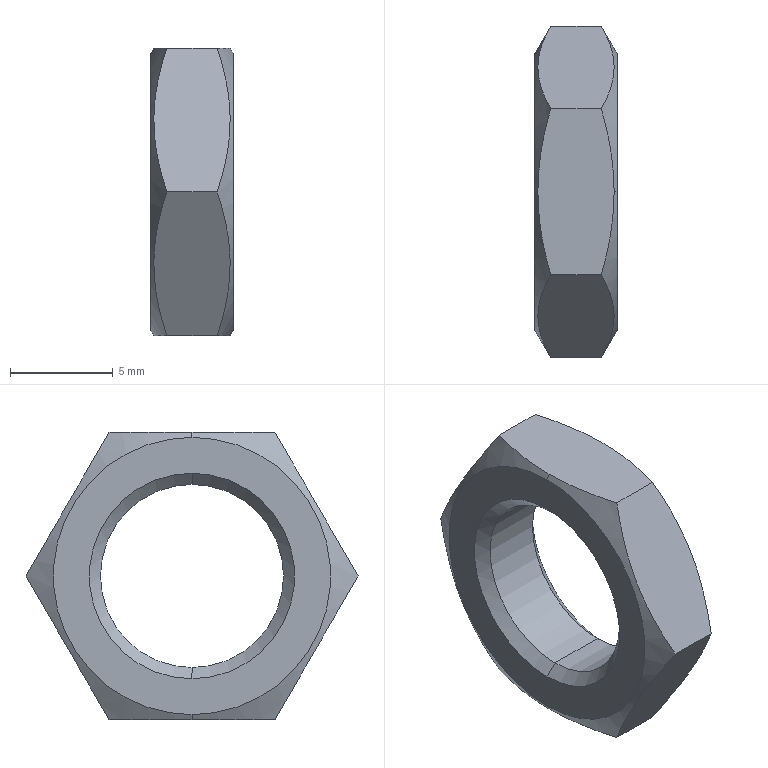Part | SolidWorks | features BaseBody 1 | 1 solid | 18 faces | box 4 x 16.166 x 14 mm | volume 408.53 mm3 | cone 8 | plane 8 | cylinder 2 | commonest cylinder face diameters 8.917 x2
STEP:
#1=CARTESIAN_POINT('',(-2.842,0.,4.458));
#2=VERTEX_POINT('',#1);
#3=CARTESIAN_POINT('',(-2.842,0.,-4.458));
#4=VERTEX_POINT('',#3);
#5=CARTESIAN_POINT('',(-2.842,0.,0.));
#6=DIRECTION('',(1.,0.,0.));
#7=DIRECTION('',(0.,1.,0.));
#8=AXIS2_PLACEMENT_3D('',#5,#6,#7);
#9=CIRCLE('',#8,4.458);
#10=EDGE_CURVE('',#2,#4,#9,.T.);
#11=ORIENTED_EDGE('',*,*,#10,.F.);
#12=CARTESIAN_POINT('',(-2.3,0.,5.));
#13=VERTEX_POINT('',#12);
#14=CARTESIAN_POINT('',(-2.3,0.,5.));
#15=DIRECTION('',(0.7071,0.,0.7071));
#16=VECTOR('',#15,1000.);
#17=LINE('',#14,#16);
#18=EDGE_CURVE('',#2,#13,#17,.T.);
#19=ORIENTED_EDGE('',*,*,#18,.T.);
#20=CARTESIAN_POINT('',(-2.3,0.,-5.));
#21=VERTEX_POINT('',#20);
#22=CARTESIAN_POINT('',(-2.3,0.,0.));
#23=DIRECTION('',(-1.,0.,0.));
#24=DIRECTION('',(0.,0.,-1.));
#25=AXIS2_PLACEMENT_3D('',#22,#23,#24);
#26=CIRCLE('',#25,5.);
#27=EDGE_CURVE('',#21,#13,#26,.T.);
#28=ORIENTED_EDGE('',*,*,#27,.F.);
#29=CARTESIAN_POINT('',(-2.3,0.,-5.));
#30=DIRECTION('',(0.7071,0.,-0.7071));
#31=VECTOR('',#30,1000.);
#32=LINE('',#29,#31);
#33=EDGE_CURVE('',#4,#21,#32,.T.);
#34=ORIENTED_EDGE('',*,*,#33,.F.);
#35=EDGE_LOOP('',(#11,#19,#28,#34));
#36=FACE_OUTER_BOUND('',#35,.T.);
#37=CARTESIAN_POINT('',(-2.3,0.,0.));
#38=DIRECTION('',(1.,0.,0.));
#39=DIRECTION('',(0.,0.,-1.));
#40=AXIS2_PLACEMENT_3D('',#37,#38,#39);
#41=CONICAL_SURFACE('',#40,5.,0.7854);
#42=ADVANCED_FACE('',(#36),#41,.F.);
#43=CARTESIAN_POINT('',(-2.3,0.,-6.75));
#44=VERTEX_POINT('',#43);
#45=CARTESIAN_POINT('',(-2.3,0.,6.75));
#46=VERTEX_POINT('',#45);
#47=CARTESIAN_POINT('',(-2.3,0.,0.));
#48=DIRECTION('',(1.,0.,0.));
#49=DIRECTION('',(0.,0.,1.));
#50=AXIS2_PLACEMENT_3D('',#47,#48,#49);
#51=CIRCLE('',#50,6.75);
#52=EDGE_CURVE('',#44,#46,#51,.T.);
#53=ORIENTED_EDGE('',*,*,#52,.F.);
#54=CARTESIAN_POINT('',(-2.444,0.,-7.));
#55=VERTEX_POINT('',#54);
#56=CARTESIAN_POINT('',(-3.074,0.,-8.091));
#57=DIRECTION('',(-0.5,0.,-0.866));
#58=VECTOR('',#57,1000.);
#59=LINE('',#56,#58);
#60=EDGE_CURVE('',#44,#55,#59,.T.);
#61=ORIENTED_EDGE('',*,*,#60,.T.);
#62=CARTESIAN_POINT('',(-3.07,4.041,-7.));
#63=VERTEX_POINT('',#62);
#64=CARTESIAN_POINT('',(-2.444,0.,-7.));
#65=CARTESIAN_POINT('',(-2.444,0.343,-7.));
#66=CARTESIAN_POINT('',(-2.459,0.6875,-7.));
#67=CARTESIAN_POINT('',(-2.516,1.369,-7.));
#68=CARTESIAN_POINT('',(-2.559,1.708,-7.));
#69=CARTESIAN_POINT('',(-2.722,2.717,-7.));
#70=CARTESIAN_POINT('',(-2.879,3.382,-7.));
#71=CARTESIAN_POINT('',(-3.07,4.041,-7.));
#72=B_SPLINE_CURVE_WITH_KNOTS('',3,(#64,#65,#66,#67,#68,#69,#70,#71),.UNSPECIFIED.,.F.,.F.,(4,2,2,4),(0.004089,0.005108,0.006126,0.008163),.UNSPECIFIED.);
#73=EDGE_CURVE('',#55,#63,#72,.T.);
#74=ORIENTED_EDGE('',*,*,#73,.T.);
#75=CARTESIAN_POINT('',(-3.07,8.083,0.));
#76=VERTEX_POINT('',#75);
#77=CARTESIAN_POINT('',(-3.07,4.041,-7.));
#78=CARTESIAN_POINT('',(-2.879,4.371,-6.429));
#79=CARTESIAN_POINT('',(-2.722,4.704,-5.853));
#80=CARTESIAN_POINT('',(-2.505,5.375,-4.69));
#81=CARTESIAN_POINT('',(-2.445,5.715,-4.102));
#82=CARTESIAN_POINT('',(-2.444,6.23,-3.209));
#83=CARTESIAN_POINT('',(-2.459,6.403,-2.91));
#84=CARTESIAN_POINT('',(-2.516,6.744,-2.319));
#85=CARTESIAN_POINT('',(-2.558,6.914,-2.025));
#86=CARTESIAN_POINT('',(-2.721,7.419,-1.149));
#87=CARTESIAN_POINT('',(-2.879,7.753,-0.5722));
#88=CARTESIAN_POINT('',(-3.07,8.083,0.));
#89=B_SPLINE_CURVE_WITH_KNOTS('',3,(#77,#78,#79,#80,#81,#82,#83,#84,#85,#86,#87,#88),.UNSPECIFIED.,.F.,.F.,(4,2,2,2,2,4),(0.,0.002041,0.004082,0.005102,0.006122,0.008163),.UNSPECIFIED.);
#90=EDGE_CURVE('',#63,#76,#89,.T.);
#91=ORIENTED_EDGE('',*,*,#90,.T.);
#92=CARTESIAN_POINT('',(-3.07,4.041,7.));
#93=VERTEX_POINT('',#92);
#94=CARTESIAN_POINT('',(-3.07,8.083,0.));
#95=CARTESIAN_POINT('',(-2.879,7.753,0.5715));
#96=CARTESIAN_POINT('',(-2.722,7.421,1.147));
#97=CARTESIAN_POINT('',(-2.505,6.749,2.31));
#98=CARTESIAN_POINT('',(-2.445,6.41,2.898));
#99=CARTESIAN_POINT('',(-2.444,5.894,3.791));
#100=CARTESIAN_POINT('',(-2.459,5.722,4.09));
#101=CARTESIAN_POINT('',(-2.516,5.38,4.681));
#102=CARTESIAN_POINT('',(-2.558,5.211,4.975));
#103=CARTESIAN_POINT('',(-2.721,4.705,5.851));
#104=CARTESIAN_POINT('',(-2.879,4.372,6.428));
#105=CARTESIAN_POINT('',(-3.07,4.041,7.));
#106=B_SPLINE_CURVE_WITH_KNOTS('',3,(#94,#95,#96,#97,#98,#99,#100,#101,#102,#103,#104,#105),.UNSPECIFIED.,.F.,.F.,(4,2,2,2,2,4),(0.,0.002041,0.004082,0.005102,0.006122,0.008163),.UNSPECIFIED.);
#107=EDGE_CURVE('',#76,#93,#106,.T.);
#108=ORIENTED_EDGE('',*,*,#107,.T.);
#109=CARTESIAN_POINT('',(-2.444,0.,7.));
#110=VERTEX_POINT('',#109);
#111=CARTESIAN_POINT('',(-3.07,4.041,7.));
#112=CARTESIAN_POINT('',(-2.879,3.38,7.));
#113=CARTESIAN_POINT('',(-2.721,2.714,7.));
#114=CARTESIAN_POINT('',(-2.504,1.369,7.));
#115=CARTESIAN_POINT('',(-2.444,0.6885,7.));
#116=CARTESIAN_POINT('',(-2.444,0.,7.));
#117=B_SPLINE_CURVE_WITH_KNOTS('',3,(#111,#112,#113,#114,#115,#116),.UNSPECIFIED.,.F.,.F.,(4,2,4),(0.,0.002045,0.004089),.UNSPECIFIED.);
#118=EDGE_CURVE('',#93,#110,#117,.T.);
#119=ORIENTED_EDGE('',*,*,#118,.T.);
#120=CARTESIAN_POINT('',(-3.074,0.,8.091));
#121=DIRECTION('',(-0.5,0.,0.866));
#122=VECTOR('',#121,1000.);
#123=LINE('',#120,#122);
#124=EDGE_CURVE('',#46,#110,#123,.T.);
#125=ORIENTED_EDGE('',*,*,#124,.F.);
#126=EDGE_LOOP('',(#53,#61,#74,#91,#108,#119,#125));
#127=FACE_OUTER_BOUND('',#126,.T.);
#128=CARTESIAN_POINT('',(-3.074,0.,0.));
#129=DIRECTION('',(-1.,0.,0.));
#130=DIRECTION('',(0.,0.,1.));
#131=AXIS2_PLACEMENT_3D('',#128,#129,#130);
#132=CONICAL_SURFACE('',#131,8.091,1.047);
#133=ADVANCED_FACE('',(#127),#132,.T.);
#134=CARTESIAN_POINT('',(-5.758,0.,4.458));
#135=VERTEX_POINT('',#134);
#136=CARTESIAN_POINT('',(-5.758,0.,-4.458));
#137=VERTEX_POINT('',#136);
#138=CARTESIAN_POINT('',(-5.758,0.,0.));
#139=DIRECTION('',(1.,0.,0.));
#140=DIRECTION('',(0.,0.,-1.));
#141=AXIS2_PLACEMENT_3D('',#138,#139,#140);
#142=CIRCLE('',#141,4.458);
#143=EDGE_CURVE('',#135,#137,#142,.T.);
#144=ORIENTED_EDGE('',*,*,#143,.F.);
#145=CARTESIAN_POINT('',(-4.3,0.,4.458));
#146=DIRECTION('',(1.,0.,0.));
#147=VECTOR('',#146,1000.);
#148=LINE('',#145,#147);
#149=EDGE_CURVE('',#135,#2,#148,.T.);
#150=ORIENTED_EDGE('',*,*,#149,.T.);
#151=ORIENTED_EDGE('',*,*,#10,.T.);
#152=CARTESIAN_POINT('',(-4.3,0.,-4.458));
#153=DIRECTION('',(1.,0.,0.));
#154=VECTOR('',#153,1000.);
#155=LINE('',#152,#154);
#156=EDGE_CURVE('',#137,#4,#155,.T.);
#157=ORIENTED_EDGE('',*,*,#156,.F.);
#158=EDGE_LOOP('',(#144,#150,#151,#157));
#159=FACE_OUTER_BOUND('',#158,.T.);
#160=CARTESIAN_POINT('',(-4.3,0.,0.));
#161=DIRECTION('',(1.,0.,0.));
#162=DIRECTION('',(0.,0.,-1.));
#163=AXIS2_PLACEMENT_3D('',#160,#161,#162);
#164=CYLINDRICAL_SURFACE('',#163,4.458);
#165=ADVANCED_FACE('',(#159),#164,.F.);
#166=ORIENTED_EDGE('',*,*,#143,.T.);
#167=CARTESIAN_POINT('',(-6.3,0.,-5.));
#168=VERTEX_POINT('',#167);
#169=CARTESIAN_POINT('',(-6.3,0.,-5.));
#170=DIRECTION('',(-0.7071,0.,-0.7071));
#171=VECTOR('',#170,1000.);
#172=LINE('',#169,#171);
#173=EDGE_CURVE('',#137,#168,#172,.T.);
#174=ORIENTED_EDGE('',*,*,#173,.T.);
#175=CARTESIAN_POINT('',(-6.3,0.,5.));
#176=VERTEX_POINT('',#175);
#177=CARTESIAN_POINT('',(-6.3,0.,0.));
#178=DIRECTION('',(1.,0.,0.));
#179=DIRECTION('',(0.,0.,1.));
#180=AXIS2_PLACEMENT_3D('',#177,#178,#179);
#181=CIRCLE('',#180,5.);
#182=EDGE_CURVE('',#176,#168,#181,.T.);
#183=ORIENTED_EDGE('',*,*,#182,.F.);
#184=CARTESIAN_POINT('',(-6.3,0.,5.));
#185=DIRECTION('',(-0.7071,0.,0.7071));
#186=VECTOR('',#185,1000.);
#187=LINE('',#184,#186);
#188=EDGE_CURVE('',#135,#176,#187,.T.);
#189=ORIENTED_EDGE('',*,*,#188,.F.);
#190=EDGE_LOOP('',(#166,#174,#183,#189));
#191=FACE_OUTER_BOUND('',#190,.T.);
#192=CARTESIAN_POINT('',(-6.3,0.,0.));
#193=DIRECTION('',(-1.,0.,0.));
#194=DIRECTION('',(0.,0.,1.));
#195=AXIS2_PLACEMENT_3D('',#192,#193,#194);
#196=CONICAL_SURFACE('',#195,5.,0.7854);
#197=ADVANCED_FACE('',(#191),#196,.F.);
#198=CARTESIAN_POINT('',(-6.3,0.,-6.75));
#199=VERTEX_POINT('',#198);
#200=CARTESIAN_POINT('',(-6.3,0.,6.75));
#201=VERTEX_POINT('',#200);
#202=CARTESIAN_POINT('',(-6.3,0.,0.));
#203=DIRECTION('',(1.,0.,0.));
#204=DIRECTION('',(0.,0.,-1.));
#205=AXIS2_PLACEMENT_3D('',#202,#203,#204);
#206=CIRCLE('',#205,6.75);
#207=EDGE_CURVE('',#199,#201,#206,.T.);
#208=ORIENTED_EDGE('',*,*,#207,.T.);
#209=CARTESIAN_POINT('',(-6.156,0.,7.));
#210=VERTEX_POINT('',#209);
#211=CARTESIAN_POINT('',(-5.526,0.,8.091));
#212=DIRECTION('',(0.5,0.,0.866));
#213=VECTOR('',#212,1000.);
#214=LINE('',#211,#213);
#215=EDGE_CURVE('',#201,#210,#214,.T.);
#216=ORIENTED_EDGE('',*,*,#215,.T.);
#217=CARTESIAN_POINT('',(-5.53,4.041,7.));
#218=VERTEX_POINT('',#217);
#219=CARTESIAN_POINT('',(-5.53,4.041,7.));
#220=CARTESIAN_POINT('',(-5.721,3.38,7.));
#221=CARTESIAN_POINT('',(-5.879,2.714,7.));
#222=CARTESIAN_POINT('',(-6.096,1.369,7.));
#223=CARTESIAN_POINT('',(-6.156,0.6885,7.));
#224=CARTESIAN_POINT('',(-6.156,0.,7.));
#225=B_SPLINE_CURVE_WITH_KNOTS('',3,(#219,#220,#221,#222,#223,#224),.UNSPECIFIED.,.F.,.F.,(4,2,4),(0.,0.002045,0.004089),.UNSPECIFIED.);
#226=EDGE_CURVE('',#218,#210,#225,.T.);
#227=ORIENTED_EDGE('',*,*,#226,.F.);
#228=CARTESIAN_POINT('',(-5.53,8.083,0.));
#229=VERTEX_POINT('',#228);
#230=CARTESIAN_POINT('',(-5.53,8.083,0.));
#231=CARTESIAN_POINT('',(-5.721,7.753,0.5715));
#232=CARTESIAN_POINT('',(-5.878,7.421,1.147));
#233=CARTESIAN_POINT('',(-6.095,6.749,2.31));
#234=CARTESIAN_POINT('',(-6.155,6.41,2.898));
#235=CARTESIAN_POINT('',(-6.156,5.894,3.791));
#236=CARTESIAN_POINT('',(-6.141,5.722,4.09));
#237=CARTESIAN_POINT('',(-6.084,5.38,4.681));
#238=CARTESIAN_POINT('',(-6.042,5.211,4.975));
#239=CARTESIAN_POINT('',(-5.879,4.705,5.851));
#240=CARTESIAN_POINT('',(-5.721,4.372,6.428));
#241=CARTESIAN_POINT('',(-5.53,4.041,7.));
#242=B_SPLINE_CURVE_WITH_KNOTS('',3,(#230,#231,#232,#233,#234,#235,#236,#237,#238,#239,#240,#241),.UNSPECIFIED.,.F.,.F.,(4,2,2,2,2,4),(0.,0.002041,0.004082,0.005102,0.006122,0.008163),.UNSPECIFIED.);
#243=EDGE_CURVE('',#229,#218,#242,.T.);
#244=ORIENTED_EDGE('',*,*,#243,.F.);
#245=CARTESIAN_POINT('',(-5.53,4.041,-7.));
#246=VERTEX_POINT('',#245);
#247=CARTESIAN_POINT('',(-5.53,4.041,-7.));
#248=CARTESIAN_POINT('',(-5.721,4.371,-6.429));
#249=CARTESIAN_POINT('',(-5.878,4.704,-5.853));
#250=CARTESIAN_POINT('',(-6.095,5.375,-4.69));
#251=CARTESIAN_POINT('',(-6.155,5.715,-4.102));
#252=CARTESIAN_POINT('',(-6.156,6.23,-3.209));
#253=CARTESIAN_POINT('',(-6.141,6.403,-2.91));
#254=CARTESIAN_POINT('',(-6.084,6.744,-2.319));
#255=CARTESIAN_POINT('',(-6.042,6.914,-2.025));
#256=CARTESIAN_POINT('',(-5.879,7.419,-1.149));
#257=CARTESIAN_POINT('',(-5.721,7.753,-0.5722));
#258=CARTESIAN_POINT('',(-5.53,8.083,0.));
#259=B_SPLINE_CURVE_WITH_KNOTS('',3,(#247,#248,#249,#250,#251,#252,#253,#254,#255,#256,#257,#258),.UNSPECIFIED.,.F.,.F.,(4,2,2,2,2,4),(0.,0.002041,0.004082,0.005102,0.006122,0.008163),.UNSPECIFIED.);
#260=EDGE_CURVE('',#246,#229,#259,.T.);
#261=ORIENTED_EDGE('',*,*,#260,.F.);
#262=CARTESIAN_POINT('',(-6.156,0.,-7.));
#263=VERTEX_POINT('',#262);
#264=CARTESIAN_POINT('',(-6.156,0.,-7.));
#265=CARTESIAN_POINT('',(-6.156,0.343,-7.));
#266=CARTESIAN_POINT('',(-6.141,0.6875,-7.));
#267=CARTESIAN_POINT('',(-6.084,1.369,-7.));
#268=CARTESIAN_POINT('',(-6.041,1.708,-7.));
#269=CARTESIAN_POINT('',(-5.878,2.717,-7.));
#270=CARTESIAN_POINT('',(-5.721,3.382,-7.));
#271=CARTESIAN_POINT('',(-5.53,4.041,-7.));
#272=B_SPLINE_CURVE_WITH_KNOTS('',3,(#264,#265,#266,#267,#268,#269,#270,#271),.UNSPECIFIED.,.F.,.F.,(4,2,2,4),(0.004089,0.005108,0.006126,0.008163),.UNSPECIFIED.);
#273=EDGE_CURVE('',#263,#246,#272,.T.);
#274=ORIENTED_EDGE('',*,*,#273,.F.);
#275=CARTESIAN_POINT('',(-5.526,0.,-8.091));
#276=DIRECTION('',(0.5,0.,-0.866));
#277=VECTOR('',#276,1000.);
#278=LINE('',#275,#277);
#279=EDGE_CURVE('',#199,#263,#278,.T.);
#280=ORIENTED_EDGE('',*,*,#279,.F.);
#281=EDGE_LOOP('',(#208,#216,#227,#244,#261,#274,#280));
#282=FACE_OUTER_BOUND('',#281,.T.);
#283=CARTESIAN_POINT('',(-5.526,0.,0.));
#284=DIRECTION('',(1.,0.,0.));
#285=DIRECTION('',(0.,0.,-1.));
#286=AXIS2_PLACEMENT_3D('',#283,#284,#285);
#287=CONICAL_SURFACE('',#286,8.091,1.047);
#288=ADVANCED_FACE('',(#282),#287,.T.);
#289=ORIENTED_EDGE('',*,*,#27,.T.);
#290=CARTESIAN_POINT('',(-2.3,0.,0.));
#291=DIRECTION('',(-1.,0.,0.));
#292=DIRECTION('',(0.,0.,-1.));
#293=AXIS2_PLACEMENT_3D('',#290,#291,#292);
#294=CIRCLE('',#293,5.);
#295=EDGE_CURVE('',#13,#21,#294,.T.);
#296=ORIENTED_EDGE('',*,*,#295,.T.);
#297=EDGE_LOOP('',(#289,#296));
#298=FACE_BOUND('',#297,.T.);
#299=CARTESIAN_POINT('',(-2.3,0.,0.));
#300=DIRECTION('',(1.,0.,0.));
#301=DIRECTION('',(0.,0.,1.));
#302=AXIS2_PLACEMENT_3D('',#299,#300,#301);
#303=CIRCLE('',#302,6.75);
#304=EDGE_CURVE('',#46,#44,#303,.T.);
#305=ORIENTED_EDGE('',*,*,#304,.T.);
#306=ORIENTED_EDGE('',*,*,#52,.T.);
#307=EDGE_LOOP('',(#305,#306));
#308=FACE_OUTER_BOUND('',#307,.T.);
#309=CARTESIAN_POINT('',(-2.3,0.,0.));
#310=DIRECTION('',(1.,0.,0.));
#311=DIRECTION('',(0.,0.,-1.));
#312=AXIS2_PLACEMENT_3D('',#309,#310,#311);
#313=PLANE('',#312);
#314=ADVANCED_FACE('',(#298,#308),#313,.T.);
#315=ORIENTED_EDGE('',*,*,#18,.F.);
#316=CARTESIAN_POINT('',(-2.842,0.,0.));
#317=DIRECTION('',(1.,0.,0.));
#318=DIRECTION('',(0.,1.,0.));
#319=AXIS2_PLACEMENT_3D('',#316,#317,#318);
#320=CIRCLE('',#319,4.458);
#321=EDGE_CURVE('',#4,#2,#320,.T.);
#322=ORIENTED_EDGE('',*,*,#321,.F.);
#323=ORIENTED_EDGE('',*,*,#33,.T.);
#324=ORIENTED_EDGE('',*,*,#295,.F.);
#325=EDGE_LOOP('',(#315,#322,#323,#324));
#326=FACE_OUTER_BOUND('',#325,.T.);
#327=CARTESIAN_POINT('',(-2.3,0.,0.));
#328=DIRECTION('',(1.,0.,0.));
#329=DIRECTION('',(0.,0.,-1.));
#330=AXIS2_PLACEMENT_3D('',#327,#328,#329);
#331=CONICAL_SURFACE('',#330,5.,0.7854);
#332=ADVANCED_FACE('',(#326),#331,.F.);
#333=ORIENTED_EDGE('',*,*,#60,.F.);
#334=ORIENTED_EDGE('',*,*,#304,.F.);
#335=ORIENTED_EDGE('',*,*,#124,.T.);
#336=CARTESIAN_POINT('',(-3.07,-4.041,7.));
#337=VERTEX_POINT('',#336);
#338=CARTESIAN_POINT('',(-2.444,0.,7.));
#339=CARTESIAN_POINT('',(-2.444,-0.343,7.));
#340=CARTESIAN_POINT('',(-2.459,-0.6875,7.));
#341=CARTESIAN_POINT('',(-2.516,-1.369,7.));
#342=CARTESIAN_POINT('',(-2.559,-1.708,7.));
#343=CARTESIAN_POINT('',(-2.722,-2.717,7.));
#344=CARTESIAN_POINT('',(-2.879,-3.382,7.));
#345=CARTESIAN_POINT('',(-3.07,-4.041,7.));
#346=B_SPLINE_CURVE_WITH_KNOTS('',3,(#338,#339,#340,#341,#342,#343,#344,#345),.UNSPECIFIED.,.F.,.F.,(4,2,2,4),(0.004089,0.005108,0.006126,0.008163),.UNSPECIFIED.);
#347=EDGE_CURVE('',#110,#337,#346,.T.);
#348=ORIENTED_EDGE('',*,*,#347,.T.);
#349=CARTESIAN_POINT('',(-3.07,-8.083,0.));
#350=VERTEX_POINT('',#349);
#351=CARTESIAN_POINT('',(-3.07,-4.041,7.));
#352=CARTESIAN_POINT('',(-2.879,-4.371,6.429));
#353=CARTESIAN_POINT('',(-2.722,-4.704,5.853));
#354=CARTESIAN_POINT('',(-2.505,-5.375,4.69));
#355=CARTESIAN_POINT('',(-2.445,-5.715,4.102));
#356=CARTESIAN_POINT('',(-2.444,-6.23,3.209));
#357=CARTESIAN_POINT('',(-2.459,-6.403,2.91));
#358=CARTESIAN_POINT('',(-2.516,-6.744,2.319));
#359=CARTESIAN_POINT('',(-2.558,-6.914,2.025));
#360=CARTESIAN_POINT('',(-2.721,-7.419,1.149));
#361=CARTESIAN_POINT('',(-2.879,-7.753,0.5722));
#362=CARTESIAN_POINT('',(-3.07,-8.083,0.));
#363=B_SPLINE_CURVE_WITH_KNOTS('',3,(#351,#352,#353,#354,#355,#356,#357,#358,#359,#360,#361,#362),.UNSPECIFIED.,.F.,.F.,(4,2,2,2,2,4),(0.,0.002041,0.004082,0.005102,0.006122,0.008163),.UNSPECIFIED.);
#364=EDGE_CURVE('',#337,#350,#363,.T.);
#365=ORIENTED_EDGE('',*,*,#364,.T.);
#366=CARTESIAN_POINT('',(-3.07,-4.041,-7.));
#367=VERTEX_POINT('',#366);
#368=CARTESIAN_POINT('',(-3.07,-8.083,0.));
#369=CARTESIAN_POINT('',(-2.879,-7.753,-0.5715));
#370=CARTESIAN_POINT('',(-2.722,-7.421,-1.147));
#371=CARTESIAN_POINT('',(-2.505,-6.749,-2.31));
#372=CARTESIAN_POINT('',(-2.445,-6.41,-2.898));
#373=CARTESIAN_POINT('',(-2.444,-5.894,-3.791));
#374=CARTESIAN_POINT('',(-2.459,-5.722,-4.09));
#375=CARTESIAN_POINT('',(-2.516,-5.38,-4.681));
#376=CARTESIAN_POINT('',(-2.558,-5.211,-4.975));
#377=CARTESIAN_POINT('',(-2.721,-4.705,-5.851));
#378=CARTESIAN_POINT('',(-2.879,-4.372,-6.428));
#379=CARTESIAN_POINT('',(-3.07,-4.041,-7.));
#380=B_SPLINE_CURVE_WITH_KNOTS('',3,(#368,#369,#370,#371,#372,#373,#374,#375,#376,#377,#378,#379),.UNSPECIFIED.,.F.,.F.,(4,2,2,2,2,4),(0.,0.002041,0.004082,0.005102,0.006122,0.008163),.UNSPECIFIED.);
#381=EDGE_CURVE('',#350,#367,#380,.T.);
#382=ORIENTED_EDGE('',*,*,#381,.T.);
#383=CARTESIAN_POINT('',(-3.07,-4.041,-7.));
#384=CARTESIAN_POINT('',(-2.879,-3.38,-7.));
#385=CARTESIAN_POINT('',(-2.721,-2.714,-7.));
#386=CARTESIAN_POINT('',(-2.504,-1.369,-7.));
#387=CARTESIAN_POINT('',(-2.444,-0.6885,-7.));
#388=CARTESIAN_POINT('',(-2.444,0.,-7.));
#389=B_SPLINE_CURVE_WITH_KNOTS('',3,(#383,#384,#385,#386,#387,#388),.UNSPECIFIED.,.F.,.F.,(4,2,4),(0.,0.002045,0.004089),.UNSPECIFIED.);
#390=EDGE_CURVE('',#367,#55,#389,.T.);
#391=ORIENTED_EDGE('',*,*,#390,.T.);
#392=EDGE_LOOP('',(#333,#334,#335,#348,#365,#382,#391));
#393=FACE_OUTER_BOUND('',#392,.T.);
#394=CARTESIAN_POINT('',(-3.074,0.,0.));
#395=DIRECTION('',(-1.,0.,0.));
#396=DIRECTION('',(0.,0.,1.));
#397=AXIS2_PLACEMENT_3D('',#394,#395,#396);
#398=CONICAL_SURFACE('',#397,8.091,1.047);
#399=ADVANCED_FACE('',(#393),#398,.T.);
#400=ORIENTED_EDGE('',*,*,#149,.F.);
#401=CARTESIAN_POINT('',(-5.758,0.,0.));
#402=DIRECTION('',(1.,0.,0.));
#403=DIRECTION('',(0.,0.,-1.));
#404=AXIS2_PLACEMENT_3D('',#401,#402,#403);
#405=CIRCLE('',#404,4.458);
#406=EDGE_CURVE('',#137,#135,#405,.T.);
#407=ORIENTED_EDGE('',*,*,#406,.F.);
#408=ORIENTED_EDGE('',*,*,#156,.T.);
#409=ORIENTED_EDGE('',*,*,#321,.T.);
#410=EDGE_LOOP('',(#400,#407,#408,#409));
#411=FACE_OUTER_BOUND('',#410,.T.);
#412=CARTESIAN_POINT('',(-4.3,0.,0.));
#413=DIRECTION('',(1.,0.,0.));
#414=DIRECTION('',(0.,0.,-1.));
#415=AXIS2_PLACEMENT_3D('',#412,#413,#414);
#416=CYLINDRICAL_SURFACE('',#415,4.458);
#417=ADVANCED_FACE('',(#411),#416,.F.);
#418=ORIENTED_EDGE('',*,*,#90,.F.);
#419=CARTESIAN_POINT('',(-2.3,4.041,-7.));
#420=DIRECTION('',(-1.,0.,0.));
#421=VECTOR('',#420,1000.);
#422=LINE('',#419,#421);
#423=EDGE_CURVE('',#63,#246,#422,.T.);
#424=ORIENTED_EDGE('',*,*,#423,.T.);
#425=ORIENTED_EDGE('',*,*,#260,.T.);
#426=CARTESIAN_POINT('',(-2.3,8.083,0.));
#427=DIRECTION('',(1.,0.,0.));
#428=VECTOR('',#427,1000.);
#429=LINE('',#426,#428);
#430=EDGE_CURVE('',#229,#76,#429,.T.);
#431=ORIENTED_EDGE('',*,*,#430,.T.);
#432=EDGE_LOOP('',(#418,#424,#425,#431));
#433=FACE_OUTER_BOUND('',#432,.T.);
#434=CARTESIAN_POINT('',(-2.3,4.041,-7.));
#435=DIRECTION('',(0.,0.866,-0.5));
#436=DIRECTION('',(0.,0.5,0.866));
#437=AXIS2_PLACEMENT_3D('',#434,#435,#436);
#438=PLANE('',#437);
#439=ADVANCED_FACE('',(#433),#438,.T.);
#440=ORIENTED_EDGE('',*,*,#390,.F.);
#441=CARTESIAN_POINT('',(-5.53,-4.041,-7.));
#442=VERTEX_POINT('',#441);
#443=CARTESIAN_POINT('',(-2.3,-4.041,-7.));
#444=DIRECTION('',(-1.,0.,0.));
#445=VECTOR('',#444,1000.);
#446=LINE('',#443,#445);
#447=EDGE_CURVE('',#367,#442,#446,.T.);
#448=ORIENTED_EDGE('',*,*,#447,.T.);
#449=CARTESIAN_POINT('',(-5.53,-4.041,-7.));
#450=CARTESIAN_POINT('',(-5.721,-3.38,-7.));
#451=CARTESIAN_POINT('',(-5.879,-2.714,-7.));
#452=CARTESIAN_POINT('',(-6.096,-1.369,-7.));
#453=CARTESIAN_POINT('',(-6.156,-0.6885,-7.));
#454=CARTESIAN_POINT('',(-6.156,0.,-7.));
#455=B_SPLINE_CURVE_WITH_KNOTS('',3,(#449,#450,#451,#452,#453,#454),.UNSPECIFIED.,.F.,.F.,(4,2,4),(0.,0.002045,0.004089),.UNSPECIFIED.);
#456=EDGE_CURVE('',#442,#263,#455,.T.);
#457=ORIENTED_EDGE('',*,*,#456,.T.);
#458=ORIENTED_EDGE('',*,*,#273,.T.);
#459=ORIENTED_EDGE('',*,*,#423,.F.);
#460=ORIENTED_EDGE('',*,*,#73,.F.);
#461=EDGE_LOOP('',(#440,#448,#457,#458,#459,#460));
#462=FACE_OUTER_BOUND('',#461,.T.);
#463=CARTESIAN_POINT('',(-2.3,-4.041,-7.));
#464=DIRECTION('',(0.,0.,-1.));
#465=DIRECTION('',(-1.,0.,0.));
#466=AXIS2_PLACEMENT_3D('',#463,#464,#465);
#467=PLANE('',#466);
#468=ADVANCED_FACE('',(#462),#467,.T.);
#469=ORIENTED_EDGE('',*,*,#381,.F.);
#470=CARTESIAN_POINT('',(-5.53,-8.083,0.));
#471=VERTEX_POINT('',#470);
#472=CARTESIAN_POINT('',(-2.3,-8.083,0.));
#473=DIRECTION('',(-1.,0.,0.));
#474=VECTOR('',#473,1000.);
#475=LINE('',#472,#474);
#476=EDGE_CURVE('',#350,#471,#475,.T.);
#477=ORIENTED_EDGE('',*,*,#476,.T.);
#478=CARTESIAN_POINT('',(-5.53,-8.083,0.));
#479=CARTESIAN_POINT('',(-5.721,-7.753,-0.5715));
#480=CARTESIAN_POINT('',(-5.878,-7.421,-1.147));
#481=CARTESIAN_POINT('',(-6.095,-6.749,-2.31));
#482=CARTESIAN_POINT('',(-6.155,-6.41,-2.898));
#483=CARTESIAN_POINT('',(-6.156,-5.894,-3.791));
#484=CARTESIAN_POINT('',(-6.141,-5.722,-4.09));
#485=CARTESIAN_POINT('',(-6.084,-5.38,-4.681));
#486=CARTESIAN_POINT('',(-6.042,-5.211,-4.975));
#487=CARTESIAN_POINT('',(-5.879,-4.705,-5.851));
#488=CARTESIAN_POINT('',(-5.721,-4.372,-6.428));
#489=CARTESIAN_POINT('',(-5.53,-4.041,-7.));
#490=B_SPLINE_CURVE_WITH_KNOTS('',3,(#478,#479,#480,#481,#482,#483,#484,#485,#486,#487,#488,#489),.UNSPECIFIED.,.F.,.F.,(4,2,2,2,2,4),(0.,0.002041,0.004082,0.005102,0.006122,0.008163),.UNSPECIFIED.);
#491=EDGE_CURVE('',#471,#442,#490,.T.);
#492=ORIENTED_EDGE('',*,*,#491,.T.);
#493=ORIENTED_EDGE('',*,*,#447,.F.);
#494=EDGE_LOOP('',(#469,#477,#492,#493));
#495=FACE_OUTER_BOUND('',#494,.T.);
#496=CARTESIAN_POINT('',(-2.3,-8.083,0.));
#497=DIRECTION('',(0.,-0.866,-0.5));
#498=DIRECTION('',(0.,0.5,-0.866));
#499=AXIS2_PLACEMENT_3D('',#496,#497,#498);
#500=PLANE('',#499);
#501=ADVANCED_FACE('',(#495),#500,.T.);
#502=ORIENTED_EDGE('',*,*,#364,.F.);
#503=CARTESIAN_POINT('',(-5.53,-4.041,7.));
#504=VERTEX_POINT('',#503);
#505=CARTESIAN_POINT('',(-2.3,-4.041,7.));
#506=DIRECTION('',(-1.,0.,0.));
#507=VECTOR('',#506,1000.);
#508=LINE('',#505,#507);
#509=EDGE_CURVE('',#337,#504,#508,.T.);
#510=ORIENTED_EDGE('',*,*,#509,.T.);
#511=CARTESIAN_POINT('',(-5.53,-4.041,7.));
#512=CARTESIAN_POINT('',(-5.721,-4.371,6.429));
#513=CARTESIAN_POINT('',(-5.878,-4.704,5.853));
#514=CARTESIAN_POINT('',(-6.095,-5.375,4.69));
#515=CARTESIAN_POINT('',(-6.155,-5.715,4.102));
#516=CARTESIAN_POINT('',(-6.156,-6.23,3.209));
#517=CARTESIAN_POINT('',(-6.141,-6.403,2.91));
#518=CARTESIAN_POINT('',(-6.084,-6.744,2.319));
#519=CARTESIAN_POINT('',(-6.042,-6.914,2.025));
#520=CARTESIAN_POINT('',(-5.879,-7.419,1.149));
#521=CARTESIAN_POINT('',(-5.721,-7.753,0.5722));
#522=CARTESIAN_POINT('',(-5.53,-8.083,0.));
#523=B_SPLINE_CURVE_WITH_KNOTS('',3,(#511,#512,#513,#514,#515,#516,#517,#518,#519,#520,#521,#522),.UNSPECIFIED.,.F.,.F.,(4,2,2,2,2,4),(0.,0.002041,0.004082,0.005102,0.006122,0.008163),.UNSPECIFIED.);
#524=EDGE_CURVE('',#504,#471,#523,.T.);
#525=ORIENTED_EDGE('',*,*,#524,.T.);
#526=ORIENTED_EDGE('',*,*,#476,.F.);
#527=EDGE_LOOP('',(#502,#510,#525,#526));
#528=FACE_OUTER_BOUND('',#527,.T.);
#529=CARTESIAN_POINT('',(-2.3,-4.041,7.));
#530=DIRECTION('',(0.,-0.866,0.5));
#531=DIRECTION('',(0.,-0.5,-0.866));
#532=AXIS2_PLACEMENT_3D('',#529,#530,#531);
#533=PLANE('',#532);
#534=ADVANCED_FACE('',(#528),#533,.T.);
#535=ORIENTED_EDGE('',*,*,#118,.F.);
#536=CARTESIAN_POINT('',(-2.3,4.041,7.));
#537=DIRECTION('',(-1.,0.,0.));
#538=VECTOR('',#537,1000.);
#539=LINE('',#536,#538);
#540=EDGE_CURVE('',#93,#218,#539,.T.);
#541=ORIENTED_EDGE('',*,*,#540,.T.);
#542=ORIENTED_EDGE('',*,*,#226,.T.);
#543=CARTESIAN_POINT('',(-6.156,0.,7.));
#544=CARTESIAN_POINT('',(-6.156,-0.343,7.));
#545=CARTESIAN_POINT('',(-6.141,-0.6875,7.));
#546=CARTESIAN_POINT('',(-6.084,-1.369,7.));
#547=CARTESIAN_POINT('',(-6.041,-1.708,7.));
#548=CARTESIAN_POINT('',(-5.878,-2.717,7.));
#549=CARTESIAN_POINT('',(-5.721,-3.382,7.));
#550=CARTESIAN_POINT('',(-5.53,-4.041,7.));
#551=B_SPLINE_CURVE_WITH_KNOTS('',3,(#543,#544,#545,#546,#547,#548,#549,#550),.UNSPECIFIED.,.F.,.F.,(4,2,2,4),(0.004089,0.005108,0.006126,0.008163),.UNSPECIFIED.);
#552=EDGE_CURVE('',#210,#504,#551,.T.);
#553=ORIENTED_EDGE('',*,*,#552,.T.);
#554=ORIENTED_EDGE('',*,*,#509,.F.);
#555=ORIENTED_EDGE('',*,*,#347,.F.);
#556=EDGE_LOOP('',(#535,#541,#542,#553,#554,#555));
#557=FACE_OUTER_BOUND('',#556,.T.);
#558=CARTESIAN_POINT('',(-2.3,4.041,7.));
#559=DIRECTION('',(0.,0.,1.));
#560=DIRECTION('',(1.,0.,0.));
#561=AXIS2_PLACEMENT_3D('',#558,#559,#560);
#562=PLANE('',#561);
#563=ADVANCED_FACE('',(#557),#562,.T.);
#564=ORIENTED_EDGE('',*,*,#107,.F.);
#565=ORIENTED_EDGE('',*,*,#430,.F.);
#566=ORIENTED_EDGE('',*,*,#243,.T.);
#567=ORIENTED_EDGE('',*,*,#540,.F.);
#568=EDGE_LOOP('',(#564,#565,#566,#567));
#569=FACE_OUTER_BOUND('',#568,.T.);
#570=CARTESIAN_POINT('',(-2.3,8.083,0.));
#571=DIRECTION('',(0.,0.866,0.5));
#572=DIRECTION('',(0.,-0.5,0.866));
#573=AXIS2_PLACEMENT_3D('',#570,#571,#572);
#574=PLANE('',#573);
#575=ADVANCED_FACE('',(#569),#574,.T.);
#576=ORIENTED_EDGE('',*,*,#173,.F.);
#577=ORIENTED_EDGE('',*,*,#406,.T.);
#578=ORIENTED_EDGE('',*,*,#188,.T.);
#579=CARTESIAN_POINT('',(-6.3,0.,0.));
#580=DIRECTION('',(1.,0.,0.));
#581=DIRECTION('',(0.,0.,1.));
#582=AXIS2_PLACEMENT_3D('',#579,#580,#581);
#583=CIRCLE('',#582,5.);
#584=EDGE_CURVE('',#168,#176,#583,.T.);
#585=ORIENTED_EDGE('',*,*,#584,.F.);
#586=EDGE_LOOP('',(#576,#577,#578,#585));
#587=FACE_OUTER_BOUND('',#586,.T.);
#588=CARTESIAN_POINT('',(-6.3,0.,0.));
#589=DIRECTION('',(-1.,0.,0.));
#590=DIRECTION('',(0.,0.,1.));
#591=AXIS2_PLACEMENT_3D('',#588,#589,#590);
#592=CONICAL_SURFACE('',#591,5.,0.7854);
#593=ADVANCED_FACE('',(#587),#592,.F.);
#594=ORIENTED_EDGE('',*,*,#215,.F.);
#595=CARTESIAN_POINT('',(-6.3,0.,0.));
#596=DIRECTION('',(1.,0.,0.));
#597=DIRECTION('',(0.,0.,-1.));
#598=AXIS2_PLACEMENT_3D('',#595,#596,#597);
#599=CIRCLE('',#598,6.75);
#600=EDGE_CURVE('',#201,#199,#599,.T.);
#601=ORIENTED_EDGE('',*,*,#600,.T.);
#602=ORIENTED_EDGE('',*,*,#279,.T.);
#603=ORIENTED_EDGE('',*,*,#456,.F.);
#604=ORIENTED_EDGE('',*,*,#491,.F.);
#605=ORIENTED_EDGE('',*,*,#524,.F.);
#606=ORIENTED_EDGE('',*,*,#552,.F.);
#607=EDGE_LOOP('',(#594,#601,#602,#603,#604,#605,#606));
#608=FACE_OUTER_BOUND('',#607,.T.);
#609=CARTESIAN_POINT('',(-5.526,0.,0.));
#610=DIRECTION('',(1.,0.,0.));
#611=DIRECTION('',(0.,0.,-1.));
#612=AXIS2_PLACEMENT_3D('',#609,#610,#611);
#613=CONICAL_SURFACE('',#612,8.091,1.047);
#614=ADVANCED_FACE('',(#608),#613,.T.);
#615=ORIENTED_EDGE('',*,*,#182,.T.);
#616=ORIENTED_EDGE('',*,*,#584,.T.);
#617=EDGE_LOOP('',(#615,#616));
#618=FACE_BOUND('',#617,.T.);
#619=ORIENTED_EDGE('',*,*,#207,.F.);
#620=ORIENTED_EDGE('',*,*,#600,.F.);
#621=EDGE_LOOP('',(#619,#620));
#622=FACE_OUTER_BOUND('',#621,.T.);
#623=CARTESIAN_POINT('',(-6.3,0.,0.));
#624=DIRECTION('',(1.,0.,0.));
#625=DIRECTION('',(0.,0.,-1.));
#626=AXIS2_PLACEMENT_3D('',#623,#624,#625);
#627=PLANE('',#626);
#628=ADVANCED_FACE('',(#618,#622),#627,.F.);
#629=CLOSED_SHELL('',(#42,#133,#165,#197,#288,#314,#332,#399,#417,#439,#468,#501,#534,#563,#575,#593,#614,#628));
#630=MANIFOLD_SOLID_BREP('',#629);
#631=CARTESIAN_POINT('',(0.,0.,0.));
#632=DIRECTION('',(0.,0.,1.));
#633=DIRECTION('',(1.,0.,0.));
#634=AXIS2_PLACEMENT_3D('',#631,#632,#633);
#635=(LENGTH_UNIT()NAMED_UNIT(*)SI_UNIT(.MILLI.,.METRE.));
#636=UNCERTAINTY_MEASURE_WITH_UNIT(LENGTH_MEASURE(0.00001),#635,'','');
#637=(NAMED_UNIT(*)PLANE_ANGLE_UNIT()SI_UNIT($,.RADIAN.));
#638=(NAMED_UNIT(*)SI_UNIT($,.STERADIAN.)SOLID_ANGLE_UNIT());
#639=(GEOMETRIC_REPRESENTATION_CONTEXT(3)GLOBAL_UNCERTAINTY_ASSIGNED_CONTEXT((#636))GLOBAL_UNIT_ASSIGNED_CONTEXT((#635,#637,#638))REPRESENTATION_CONTEXT('',''));
#640=ADVANCED_BREP_SHAPE_REPRESENTATION('',(#630,#634),#639);